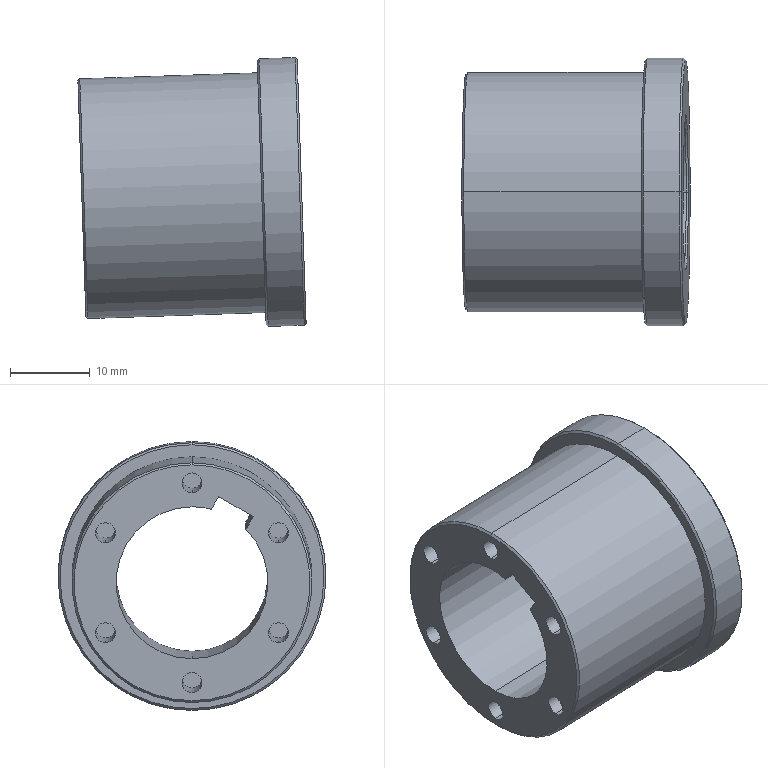Part | STEP file | 2026.6.15-Main Assembly图.sldasm-Part-99 | 1 solid | 40 faces | box 28.541 x 33.5 x 33.633 mm | volume 11781 mm3 | cylinder 19 | plane 12 | cone 9 | commonest cylinder face diameters 2.5 x12 19 x3 30 x2 33.5 x2
STEP:
#1=CARTESIAN_POINT('',(-1536.134,735.086,4103.375));
#2=VERTEX_POINT('',#1);
#3=CARTESIAN_POINT('',(-1537.25,735.086,4136.356));
#4=VERTEX_POINT('',#3);
#5=CARTESIAN_POINT('',(-1536.692,735.086,4119.866));
#6=DIRECTION('',(0.9994,0.,0.03381));
#7=DIRECTION('',(0.03381,0.,-0.9994));
#8=AXIS2_PLACEMENT_3D('',#5,#6,#7);
#9=CIRCLE('',#8,16.5);
#10=EDGE_CURVE('',#2,#4,#9,.T.);
#11=ORIENTED_EDGE('',*,*,#10,.F.);
#12=CARTESIAN_POINT('',(-1536.375,735.086,4103.117));
#13=VERTEX_POINT('',#12);
#14=CARTESIAN_POINT('',(-1536.134,735.086,4103.375));
#15=DIRECTION('',(-0.6828,0.,-0.7306));
#16=VECTOR('',#15,1000.);
#17=LINE('',#14,#16);
#18=EDGE_CURVE('',#2,#13,#17,.T.);
#19=ORIENTED_EDGE('',*,*,#18,.T.);
#20=CARTESIAN_POINT('',(-1537.508,735.086,4136.598));
#21=VERTEX_POINT('',#20);
#22=CARTESIAN_POINT('',(-1536.941,735.086,4119.857));
#23=DIRECTION('',(-0.9994,0.,-0.03381));
#24=DIRECTION('',(0.03381,0.,-0.9994));
#25=AXIS2_PLACEMENT_3D('',#22,#23,#24);
#26=CIRCLE('',#25,16.75);
#27=EDGE_CURVE('',#21,#13,#26,.T.);
#28=ORIENTED_EDGE('',*,*,#27,.F.);
#29=CARTESIAN_POINT('',(-1537.25,735.086,4136.356));
#30=DIRECTION('',(-0.7306,0.,0.6828));
#31=VECTOR('',#30,1000.);
#32=LINE('',#29,#31);
#33=EDGE_CURVE('',#4,#21,#32,.T.);
#34=ORIENTED_EDGE('',*,*,#33,.F.);
#35=EDGE_LOOP('',(#11,#19,#28,#34));
#36=FACE_OUTER_BOUND('',#35,.T.);
#37=CARTESIAN_POINT('',(-1536.692,735.086,4119.866));
#38=DIRECTION('',(-0.9994,0.,-0.03381));
#39=DIRECTION('',(-0.03381,0.,0.9994));
#40=AXIS2_PLACEMENT_3D('',#37,#38,#39);
#41=CONICAL_SURFACE('',#40,16.5,0.7854);
#42=ADVANCED_FACE('',(#36),#41,.T.);
#43=CARTESIAN_POINT('',(-1542.247,735.086,4136.187));
#44=VERTEX_POINT('',#43);
#45=CARTESIAN_POINT('',(-1541.131,735.086,4103.206));
#46=VERTEX_POINT('',#45);
#47=CARTESIAN_POINT('',(-1541.689,735.086,4119.697));
#48=DIRECTION('',(-0.9994,0.,-0.03381));
#49=DIRECTION('',(0.03381,0.,-0.9994));
#50=AXIS2_PLACEMENT_3D('',#47,#48,#49);
#51=CIRCLE('',#50,16.5);
#52=EDGE_CURVE('',#44,#46,#51,.T.);
#53=ORIENTED_EDGE('',*,*,#52,.F.);
#54=CARTESIAN_POINT('',(-1542.005,735.086,4136.445));
#55=VERTEX_POINT('',#54);
#56=CARTESIAN_POINT('',(-1542.005,735.086,4136.445));
#57=DIRECTION('',(0.6828,0.,0.7306));
#58=VECTOR('',#57,1000.);
#59=LINE('',#56,#58);
#60=EDGE_CURVE('',#44,#55,#59,.T.);
#61=ORIENTED_EDGE('',*,*,#60,.T.);
#62=CARTESIAN_POINT('',(-1540.873,735.086,4102.965));
#63=VERTEX_POINT('',#62);
#64=CARTESIAN_POINT('',(-1541.439,735.086,4119.705));
#65=DIRECTION('',(0.9994,0.,0.03381));
#66=DIRECTION('',(0.03381,0.,-0.9994));
#67=AXIS2_PLACEMENT_3D('',#64,#65,#66);
#68=CIRCLE('',#67,16.75);
#69=EDGE_CURVE('',#63,#55,#68,.T.);
#70=ORIENTED_EDGE('',*,*,#69,.F.);
#71=CARTESIAN_POINT('',(-1540.873,735.086,4102.965));
#72=DIRECTION('',(0.7306,0.,-0.6828));
#73=VECTOR('',#72,1000.);
#74=LINE('',#71,#73);
#75=EDGE_CURVE('',#46,#63,#74,.T.);
#76=ORIENTED_EDGE('',*,*,#75,.F.);
#77=EDGE_LOOP('',(#53,#61,#70,#76));
#78=FACE_OUTER_BOUND('',#77,.T.);
#79=CARTESIAN_POINT('',(-1541.439,735.086,4119.705));
#80=DIRECTION('',(0.9994,0.,0.03381));
#81=DIRECTION('',(0.03381,0.,-0.9994));
#82=AXIS2_PLACEMENT_3D('',#79,#80,#81);
#83=CONICAL_SURFACE('',#82,16.75,0.7854);
#84=ADVANCED_FACE('',(#78),#83,.T.);
#85=CARTESIAN_POINT('',(-1537.263,735.086,4129.352));
#86=VERTEX_POINT('',#85);
#87=CARTESIAN_POINT('',(-1537.252,732.668,4129.039));
#88=VERTEX_POINT('',#87);
#89=CARTESIAN_POINT('',(-1536.941,735.086,4119.857));
#90=DIRECTION('',(0.9994,0.,0.03381));
#91=DIRECTION('',(0.03381,0.,-0.9994));
#92=AXIS2_PLACEMENT_3D('',#89,#90,#91);
#93=CIRCLE('',#92,9.5);
#94=EDGE_CURVE('',#86,#88,#93,.T.);
#95=ORIENTED_EDGE('',*,*,#94,.F.);
#96=CARTESIAN_POINT('',(-1537.021,735.086,4129.61));
#97=VERTEX_POINT('',#96);
#98=CARTESIAN_POINT('',(-1537.263,735.086,4129.352));
#99=DIRECTION('',(0.6828,0.,0.7306));
#100=VECTOR('',#99,1000.);
#101=LINE('',#98,#100);
#102=EDGE_CURVE('',#86,#97,#101,.T.);
#103=ORIENTED_EDGE('',*,*,#102,.T.);
#104=CARTESIAN_POINT('',(-1537.01,732.539,4129.272));
#105=VERTEX_POINT('',#104);
#106=CARTESIAN_POINT('',(-1536.692,735.086,4119.866));
#107=DIRECTION('',(-0.9994,0.,-0.03381));
#108=DIRECTION('',(0.03381,0.,-0.9994));
#109=AXIS2_PLACEMENT_3D('',#106,#107,#108);
#110=CIRCLE('',#109,9.75);
#111=EDGE_CURVE('',#105,#97,#110,.T.);
#112=ORIENTED_EDGE('',*,*,#111,.F.);
#113=CARTESIAN_POINT('',(-1537.252,732.668,4129.039));
#114=CARTESIAN_POINT('',(-1537.171,732.625,4129.117));
#115=CARTESIAN_POINT('',(-1537.091,732.582,4129.194));
#116=CARTESIAN_POINT('',(-1537.01,732.539,4129.272));
#117=B_SPLINE_CURVE_WITH_KNOTS('',3,(#113,#114,#115,#116),.UNSPECIFIED.,.F.,.F.,(4,4),(0.,0.0003599),.UNSPECIFIED.);
#118=EDGE_CURVE('',#88,#105,#117,.T.);
#119=ORIENTED_EDGE('',*,*,#118,.F.);
#120=EDGE_LOOP('',(#95,#103,#112,#119));
#121=FACE_OUTER_BOUND('',#120,.T.);
#122=CARTESIAN_POINT('',(-1536.941,735.086,4119.857));
#123=DIRECTION('',(0.9994,0.,0.03381));
#124=DIRECTION('',(0.03381,0.,-0.9994));
#125=AXIS2_PLACEMENT_3D('',#122,#123,#124);
#126=CONICAL_SURFACE('',#125,9.5,0.7854);
#127=ADVANCED_FACE('',(#121),#126,.F.);
#128=ORIENTED_EDGE('',*,*,#102,.F.);
#129=CARTESIAN_POINT('',(-1536.62,735.086,4110.363));
#130=VERTEX_POINT('',#129);
#131=CARTESIAN_POINT('',(-1536.941,735.086,4119.857));
#132=DIRECTION('',(0.9994,0.,0.03381));
#133=DIRECTION('',(0.03381,0.,-0.9994));
#134=AXIS2_PLACEMENT_3D('',#131,#132,#133);
#135=CIRCLE('',#134,9.5);
#136=EDGE_CURVE('',#130,#86,#135,.T.);
#137=ORIENTED_EDGE('',*,*,#136,.F.);
#138=CARTESIAN_POINT('',(-1536.362,735.086,4110.121));
#139=VERTEX_POINT('',#138);
#140=CARTESIAN_POINT('',(-1536.62,735.086,4110.363));
#141=DIRECTION('',(0.7306,0.,-0.6828));
#142=VECTOR('',#141,1000.);
#143=LINE('',#140,#142);
#144=EDGE_CURVE('',#130,#139,#143,.T.);
#145=ORIENTED_EDGE('',*,*,#144,.T.);
#146=CARTESIAN_POINT('',(-1536.692,735.086,4119.866));
#147=DIRECTION('',(-0.9994,0.,-0.03381));
#148=DIRECTION('',(0.03381,0.,-0.9994));
#149=AXIS2_PLACEMENT_3D('',#146,#147,#148);
#150=CIRCLE('',#149,9.75);
#151=EDGE_CURVE('',#97,#139,#150,.T.);
#152=ORIENTED_EDGE('',*,*,#151,.F.);
#153=EDGE_LOOP('',(#128,#137,#145,#152));
#154=FACE_OUTER_BOUND('',#153,.T.);
#155=CARTESIAN_POINT('',(-1536.941,735.086,4119.857));
#156=DIRECTION('',(0.9994,0.,0.03381));
#157=DIRECTION('',(0.03381,0.,-0.9994));
#158=AXIS2_PLACEMENT_3D('',#155,#156,#157);
#159=CONICAL_SURFACE('',#158,9.5,0.7854);
#160=ADVANCED_FACE('',(#154),#159,.F.);
#161=CARTESIAN_POINT('',(-1564.675,735.086,4133.677));
#162=VERTEX_POINT('',#161);
#163=CARTESIAN_POINT('',(-1563.677,735.086,4104.194));
#164=VERTEX_POINT('',#163);
#165=CARTESIAN_POINT('',(-1564.176,735.086,4118.936));
#166=DIRECTION('',(-0.9994,0.,-0.03381));
#167=DIRECTION('',(0.03381,0.,-0.9994));
#168=AXIS2_PLACEMENT_3D('',#165,#166,#167);
#169=CIRCLE('',#168,14.75);
#170=EDGE_CURVE('',#162,#164,#169,.T.);
#171=ORIENTED_EDGE('',*,*,#170,.F.);
#172=CARTESIAN_POINT('',(-1564.433,735.086,4133.936));
#173=VERTEX_POINT('',#172);
#174=CARTESIAN_POINT('',(-1564.433,735.086,4133.936));
#175=DIRECTION('',(0.6828,0.,0.7306));
#176=VECTOR('',#175,1000.);
#177=LINE('',#174,#176);
#178=EDGE_CURVE('',#162,#173,#177,.T.);
#179=ORIENTED_EDGE('',*,*,#178,.T.);
#180=CARTESIAN_POINT('',(-1563.419,735.086,4103.953));
#181=VERTEX_POINT('',#180);
#182=CARTESIAN_POINT('',(-1563.926,735.086,4118.944));
#183=DIRECTION('',(0.9994,0.,0.03381));
#184=DIRECTION('',(0.03381,0.,-0.9994));
#185=AXIS2_PLACEMENT_3D('',#182,#183,#184);
#186=CIRCLE('',#185,15.);
#187=EDGE_CURVE('',#181,#173,#186,.T.);
#188=ORIENTED_EDGE('',*,*,#187,.F.);
#189=CARTESIAN_POINT('',(-1563.419,735.086,4103.953));
#190=DIRECTION('',(0.7306,0.,-0.6828));
#191=VECTOR('',#190,1000.);
#192=LINE('',#189,#191);
#193=EDGE_CURVE('',#164,#181,#192,.T.);
#194=ORIENTED_EDGE('',*,*,#193,.F.);
#195=EDGE_LOOP('',(#171,#179,#188,#194));
#196=FACE_OUTER_BOUND('',#195,.T.);
#197=CARTESIAN_POINT('',(-1563.926,735.086,4118.944));
#198=DIRECTION('',(0.9994,0.,0.03381));
#199=DIRECTION('',(0.03381,0.,-0.9994));
#200=AXIS2_PLACEMENT_3D('',#197,#198,#199);
#201=CONICAL_SURFACE('',#200,15.,0.7854);
#202=ADVANCED_FACE('',(#196),#201,.T.);
#203=CARTESIAN_POINT('',(-1564.556,735.086,4130.179));
#204=VERTEX_POINT('',#203);
#205=CARTESIAN_POINT('',(-1564.641,735.086,4132.678));
#206=VERTEX_POINT('',#205);
#207=CARTESIAN_POINT('',(-1564.599,735.086,4131.429));
#208=DIRECTION('',(-0.9994,0.,-0.03381));
#209=DIRECTION('',(-0.02928,-0.5,0.8655));
#210=AXIS2_PLACEMENT_3D('',#207,#208,#209);
#211=CIRCLE('',#210,1.25);
#212=EDGE_CURVE('',#204,#206,#211,.T.);
#213=ORIENTED_EDGE('',*,*,#212,.T.);
#214=CARTESIAN_POINT('',(-1547.651,735.086,4133.253));
#215=VERTEX_POINT('',#214);
#216=CARTESIAN_POINT('',(-1564.641,735.086,4132.678));
#217=DIRECTION('',(0.9994,0.,0.03381));
#218=VECTOR('',#217,1000.);
#219=LINE('',#216,#218);
#220=EDGE_CURVE('',#206,#215,#219,.T.);
#221=ORIENTED_EDGE('',*,*,#220,.T.);
#222=CARTESIAN_POINT('',(-1547.566,735.086,4130.754));
#223=VERTEX_POINT('',#222);
#224=CARTESIAN_POINT('',(-1547.608,735.086,4132.003));
#225=DIRECTION('',(0.9994,0.,0.03381));
#226=DIRECTION('',(-0.02928,-0.5,0.8655));
#227=AXIS2_PLACEMENT_3D('',#224,#225,#226);
#228=CIRCLE('',#227,1.25);
#229=EDGE_CURVE('',#215,#223,#228,.T.);
#230=ORIENTED_EDGE('',*,*,#229,.T.);
#231=CARTESIAN_POINT('',(-1564.556,735.086,4130.179));
#232=DIRECTION('',(0.9994,0.,0.03381));
#233=VECTOR('',#232,1000.);
#234=LINE('',#231,#233);
#235=EDGE_CURVE('',#204,#223,#234,.T.);
#236=ORIENTED_EDGE('',*,*,#235,.F.);
#237=EDGE_LOOP('',(#213,#221,#230,#236));
#238=FACE_OUTER_BOUND('',#237,.T.);
#239=CARTESIAN_POINT('',(-1564.599,735.086,4131.429));
#240=DIRECTION('',(0.9994,0.,0.03381));
#241=DIRECTION('',(0.03381,0.,-0.9994));
#242=AXIS2_PLACEMENT_3D('',#239,#240,#241);
#243=CYLINDRICAL_SURFACE('',#242,1.25);
#244=ADVANCED_FACE('',(#238),#243,.F.);
#245=CARTESIAN_POINT('',(-1564.345,724.26,4123.933));
#246=VERTEX_POINT('',#245);
#247=CARTESIAN_POINT('',(-1564.429,724.26,4126.431));
#248=VERTEX_POINT('',#247);
#249=CARTESIAN_POINT('',(-1564.387,724.26,4125.182));
#250=DIRECTION('',(-0.9994,0.,-0.03381));
#251=DIRECTION('',(-0.02928,-0.5,0.8655));
#252=AXIS2_PLACEMENT_3D('',#249,#250,#251);
#253=CIRCLE('',#252,1.25);
#254=EDGE_CURVE('',#246,#248,#253,.T.);
#255=ORIENTED_EDGE('',*,*,#254,.T.);
#256=CARTESIAN_POINT('',(-1547.439,724.26,4127.006));
#257=VERTEX_POINT('',#256);
#258=CARTESIAN_POINT('',(-1564.429,724.26,4126.431));
#259=DIRECTION('',(0.9994,0.,0.03381));
#260=VECTOR('',#259,1000.);
#261=LINE('',#258,#260);
#262=EDGE_CURVE('',#248,#257,#261,.T.);
#263=ORIENTED_EDGE('',*,*,#262,.T.);
#264=CARTESIAN_POINT('',(-1547.355,724.26,4124.508));
#265=VERTEX_POINT('',#264);
#266=CARTESIAN_POINT('',(-1547.397,724.26,4125.757));
#267=DIRECTION('',(0.9994,0.,0.03381));
#268=DIRECTION('',(-0.02928,-0.5,0.8655));
#269=AXIS2_PLACEMENT_3D('',#266,#267,#268);
#270=CIRCLE('',#269,1.25);
#271=EDGE_CURVE('',#257,#265,#270,.T.);
#272=ORIENTED_EDGE('',*,*,#271,.T.);
#273=CARTESIAN_POINT('',(-1564.345,724.26,4123.933));
#274=DIRECTION('',(0.9994,0.,0.03381));
#275=VECTOR('',#274,1000.);
#276=LINE('',#273,#275);
#277=EDGE_CURVE('',#246,#265,#276,.T.);
#278=ORIENTED_EDGE('',*,*,#277,.F.);
#279=EDGE_LOOP('',(#255,#263,#272,#278));
#280=FACE_OUTER_BOUND('',#279,.T.);
#281=CARTESIAN_POINT('',(-1564.387,724.26,4125.182));
#282=DIRECTION('',(0.9994,0.,0.03381));
#283=DIRECTION('',(0.03381,0.,-0.9994));
#284=AXIS2_PLACEMENT_3D('',#281,#282,#283);
#285=CYLINDRICAL_SURFACE('',#284,1.25);
#286=ADVANCED_FACE('',(#280),#285,.F.);
#287=CARTESIAN_POINT('',(-1563.922,724.26,4111.44));
#288=VERTEX_POINT('',#287);
#289=CARTESIAN_POINT('',(-1564.007,724.26,4113.939));
#290=VERTEX_POINT('',#289);
#291=CARTESIAN_POINT('',(-1563.965,724.26,4112.689));
#292=DIRECTION('',(-0.9994,0.,-0.03381));
#293=DIRECTION('',(-0.02928,-0.5,0.8655));
#294=AXIS2_PLACEMENT_3D('',#291,#292,#293);
#295=CIRCLE('',#294,1.25);
#296=EDGE_CURVE('',#288,#290,#295,.T.);
#297=ORIENTED_EDGE('',*,*,#296,.T.);
#298=CARTESIAN_POINT('',(-1547.017,724.26,4114.513));
#299=VERTEX_POINT('',#298);
#300=CARTESIAN_POINT('',(-1564.007,724.26,4113.939));
#301=DIRECTION('',(0.9994,0.,0.03381));
#302=VECTOR('',#301,1000.);
#303=LINE('',#300,#302);
#304=EDGE_CURVE('',#290,#299,#303,.T.);
#305=ORIENTED_EDGE('',*,*,#304,.T.);
#306=CARTESIAN_POINT('',(-1546.932,724.26,4112.015));
#307=VERTEX_POINT('',#306);
#308=CARTESIAN_POINT('',(-1546.974,724.26,4113.264));
#309=DIRECTION('',(0.9994,0.,0.03381));
#310=DIRECTION('',(-0.02928,-0.5,0.8655));
#311=AXIS2_PLACEMENT_3D('',#308,#309,#310);
#312=CIRCLE('',#311,1.25);
#313=EDGE_CURVE('',#299,#307,#312,.T.);
#314=ORIENTED_EDGE('',*,*,#313,.T.);
#315=CARTESIAN_POINT('',(-1563.922,724.26,4111.44));
#316=DIRECTION('',(0.9994,0.,0.03381));
#317=VECTOR('',#316,1000.);
#318=LINE('',#315,#317);
#319=EDGE_CURVE('',#288,#307,#318,.T.);
#320=ORIENTED_EDGE('',*,*,#319,.F.);
#321=EDGE_LOOP('',(#297,#305,#314,#320));
#322=FACE_OUTER_BOUND('',#321,.T.);
#323=CARTESIAN_POINT('',(-1563.965,724.26,4112.689));
#324=DIRECTION('',(0.9994,0.,0.03381));
#325=DIRECTION('',(0.03381,0.,-0.9994));
#326=AXIS2_PLACEMENT_3D('',#323,#324,#325);
#327=CYLINDRICAL_SURFACE('',#326,1.25);
#328=ADVANCED_FACE('',(#322),#327,.F.);
#329=CARTESIAN_POINT('',(-1563.711,735.086,4105.194));
#330=VERTEX_POINT('',#329);
#331=CARTESIAN_POINT('',(-1563.795,735.086,4107.692));
#332=VERTEX_POINT('',#331);
#333=CARTESIAN_POINT('',(-1563.753,735.086,4106.443));
#334=DIRECTION('',(-0.9994,0.,-0.03381));
#335=DIRECTION('',(-0.02928,-0.5,0.8655));
#336=AXIS2_PLACEMENT_3D('',#333,#334,#335);
#337=CIRCLE('',#336,1.25);
#338=EDGE_CURVE('',#330,#332,#337,.T.);
#339=ORIENTED_EDGE('',*,*,#338,.T.);
#340=CARTESIAN_POINT('',(-1546.805,735.086,4108.267));
#341=VERTEX_POINT('',#340);
#342=CARTESIAN_POINT('',(-1563.795,735.086,4107.692));
#343=DIRECTION('',(0.9994,0.,0.03381));
#344=VECTOR('',#343,1000.);
#345=LINE('',#342,#344);
#346=EDGE_CURVE('',#332,#341,#345,.T.);
#347=ORIENTED_EDGE('',*,*,#346,.T.);
#348=CARTESIAN_POINT('',(-1546.721,735.086,4105.768));
#349=VERTEX_POINT('',#348);
#350=CARTESIAN_POINT('',(-1546.763,735.086,4107.018));
#351=DIRECTION('',(0.9994,0.,0.03381));
#352=DIRECTION('',(-0.02928,-0.5,0.8655));
#353=AXIS2_PLACEMENT_3D('',#350,#351,#352);
#354=CIRCLE('',#353,1.25);
#355=EDGE_CURVE('',#341,#349,#354,.T.);
#356=ORIENTED_EDGE('',*,*,#355,.T.);
#357=CARTESIAN_POINT('',(-1563.711,735.086,4105.194));
#358=DIRECTION('',(0.9994,0.,0.03381));
#359=VECTOR('',#358,1000.);
#360=LINE('',#357,#359);
#361=EDGE_CURVE('',#330,#349,#360,.T.);
#362=ORIENTED_EDGE('',*,*,#361,.F.);
#363=EDGE_LOOP('',(#339,#347,#356,#362));
#364=FACE_OUTER_BOUND('',#363,.T.);
#365=CARTESIAN_POINT('',(-1563.753,735.086,4106.443));
#366=DIRECTION('',(0.9994,0.,0.03381));
#367=DIRECTION('',(0.03381,0.,-0.9994));
#368=AXIS2_PLACEMENT_3D('',#365,#366,#367);
#369=CYLINDRICAL_SURFACE('',#368,1.25);
#370=ADVANCED_FACE('',(#364),#369,.F.);
#371=CARTESIAN_POINT('',(-1563.922,745.911,4111.44));
#372=VERTEX_POINT('',#371);
#373=CARTESIAN_POINT('',(-1564.007,745.911,4113.939));
#374=VERTEX_POINT('',#373);
#375=CARTESIAN_POINT('',(-1563.965,745.911,4112.689));
#376=DIRECTION('',(-0.9994,0.,-0.03381));
#377=DIRECTION('',(-0.02928,-0.5,0.8655));
#378=AXIS2_PLACEMENT_3D('',#375,#376,#377);
#379=CIRCLE('',#378,1.25);
#380=EDGE_CURVE('',#372,#374,#379,.T.);
#381=ORIENTED_EDGE('',*,*,#380,.T.);
#382=CARTESIAN_POINT('',(-1547.017,745.911,4114.513));
#383=VERTEX_POINT('',#382);
#384=CARTESIAN_POINT('',(-1564.007,745.911,4113.939));
#385=DIRECTION('',(0.9994,0.,0.03381));
#386=VECTOR('',#385,1000.);
#387=LINE('',#384,#386);
#388=EDGE_CURVE('',#374,#383,#387,.T.);
#389=ORIENTED_EDGE('',*,*,#388,.T.);
#390=CARTESIAN_POINT('',(-1546.932,745.911,4112.015));
#391=VERTEX_POINT('',#390);
#392=CARTESIAN_POINT('',(-1546.974,745.911,4113.264));
#393=DIRECTION('',(0.9994,0.,0.03381));
#394=DIRECTION('',(-0.02928,-0.5,0.8655));
#395=AXIS2_PLACEMENT_3D('',#392,#393,#394);
#396=CIRCLE('',#395,1.25);
#397=EDGE_CURVE('',#383,#391,#396,.T.);
#398=ORIENTED_EDGE('',*,*,#397,.T.);
#399=CARTESIAN_POINT('',(-1563.922,745.911,4111.44));
#400=DIRECTION('',(0.9994,0.,0.03381));
#401=VECTOR('',#400,1000.);
#402=LINE('',#399,#401);
#403=EDGE_CURVE('',#372,#391,#402,.T.);
#404=ORIENTED_EDGE('',*,*,#403,.F.);
#405=EDGE_LOOP('',(#381,#389,#398,#404));
#406=FACE_OUTER_BOUND('',#405,.T.);
#407=CARTESIAN_POINT('',(-1563.965,745.911,4112.689));
#408=DIRECTION('',(0.9994,0.,0.03381));
#409=DIRECTION('',(0.03381,0.,-0.9994));
#410=AXIS2_PLACEMENT_3D('',#407,#408,#409);
#411=CYLINDRICAL_SURFACE('',#410,1.25);
#412=ADVANCED_FACE('',(#406),#411,.F.);
#413=CARTESIAN_POINT('',(-1564.345,745.911,4123.933));
#414=VERTEX_POINT('',#413);
#415=CARTESIAN_POINT('',(-1564.429,745.911,4126.431));
#416=VERTEX_POINT('',#415);
#417=CARTESIAN_POINT('',(-1564.387,745.911,4125.182));
#418=DIRECTION('',(-0.9994,0.,-0.03381));
#419=DIRECTION('',(-0.02928,-0.5,0.8655));
#420=AXIS2_PLACEMENT_3D('',#417,#418,#419);
#421=CIRCLE('',#420,1.25);
#422=EDGE_CURVE('',#414,#416,#421,.T.);
#423=ORIENTED_EDGE('',*,*,#422,.T.);
#424=CARTESIAN_POINT('',(-1547.439,745.911,4127.006));
#425=VERTEX_POINT('',#424);
#426=CARTESIAN_POINT('',(-1564.429,745.911,4126.431));
#427=DIRECTION('',(0.9994,0.,0.03381));
#428=VECTOR('',#427,1000.);
#429=LINE('',#426,#428);
#430=EDGE_CURVE('',#416,#425,#429,.T.);
#431=ORIENTED_EDGE('',*,*,#430,.T.);
#432=CARTESIAN_POINT('',(-1547.355,745.911,4124.508));
#433=VERTEX_POINT('',#432);
#434=CARTESIAN_POINT('',(-1547.397,745.911,4125.757));
#435=DIRECTION('',(0.9994,0.,0.03381));
#436=DIRECTION('',(-0.02928,-0.5,0.8655));
#437=AXIS2_PLACEMENT_3D('',#434,#435,#436);
#438=CIRCLE('',#437,1.25);
#439=EDGE_CURVE('',#425,#433,#438,.T.);
#440=ORIENTED_EDGE('',*,*,#439,.T.);
#441=CARTESIAN_POINT('',(-1564.345,745.911,4123.933));
#442=DIRECTION('',(0.9994,0.,0.03381));
#443=VECTOR('',#442,1000.);
#444=LINE('',#441,#443);
#445=EDGE_CURVE('',#414,#433,#444,.T.);
#446=ORIENTED_EDGE('',*,*,#445,.F.);
#447=EDGE_LOOP('',(#423,#431,#440,#446));
#448=FACE_OUTER_BOUND('',#447,.T.);
#449=CARTESIAN_POINT('',(-1564.387,745.911,4125.182));
#450=DIRECTION('',(0.9994,0.,0.03381));
#451=DIRECTION('',(0.03381,0.,-0.9994));
#452=AXIS2_PLACEMENT_3D('',#449,#450,#451);
#453=CYLINDRICAL_SURFACE('',#452,1.25);
#454=ADVANCED_FACE('',(#448),#453,.F.);
#455=CARTESIAN_POINT('',(-1564.497,735.086,4128.43));
#456=VERTEX_POINT('',#455);
#457=CARTESIAN_POINT('',(-1564.487,732.668,4128.118));
#458=VERTEX_POINT('',#457);
#459=CARTESIAN_POINT('',(-1564.176,735.086,4118.936));
#460=DIRECTION('',(0.9994,0.,0.03381));
#461=DIRECTION('',(-0.01691,0.866,0.4997));
#462=AXIS2_PLACEMENT_3D('',#459,#460,#461);
#463=CIRCLE('',#462,9.5);
#464=EDGE_CURVE('',#456,#458,#463,.T.);
#465=ORIENTED_EDGE('',*,*,#464,.F.);
#466=CARTESIAN_POINT('',(-1564.497,735.086,4128.43));
#467=DIRECTION('',(0.9994,0.,0.03381));
#468=VECTOR('',#467,1000.);
#469=LINE('',#466,#468);
#470=EDGE_CURVE('',#456,#86,#469,.T.);
#471=ORIENTED_EDGE('',*,*,#470,.T.);
#472=ORIENTED_EDGE('',*,*,#94,.T.);
#473=CARTESIAN_POINT('',(-1564.487,732.668,4128.118));
#474=DIRECTION('',(-0.9994,0.,-0.03381));
#475=VECTOR('',#474,1000.);
#476=LINE('',#473,#475);
#477=EDGE_CURVE('',#88,#458,#476,.T.);
#478=ORIENTED_EDGE('',*,*,#477,.T.);
#479=EDGE_LOOP('',(#465,#471,#472,#478));
#480=FACE_OUTER_BOUND('',#479,.T.);
#481=CARTESIAN_POINT('',(-1564.176,735.086,4118.936));
#482=DIRECTION('',(0.9994,0.,0.03381));
#483=DIRECTION('',(0.03381,0.,-0.9994));
#484=AXIS2_PLACEMENT_3D('',#481,#482,#483);
#485=CYLINDRICAL_SURFACE('',#484,9.5);
#486=ADVANCED_FACE('',(#480),#485,.F.);
#487=ORIENTED_EDGE('',*,*,#470,.F.);
#488=CARTESIAN_POINT('',(-1563.855,735.086,4109.441));
#489=VERTEX_POINT('',#488);
#490=CARTESIAN_POINT('',(-1564.176,735.086,4118.936));
#491=DIRECTION('',(0.9994,0.,0.03381));
#492=DIRECTION('',(-0.01691,0.866,0.4997));
#493=AXIS2_PLACEMENT_3D('',#490,#491,#492);
#494=CIRCLE('',#493,9.5);
#495=EDGE_CURVE('',#489,#456,#494,.T.);
#496=ORIENTED_EDGE('',*,*,#495,.F.);
#497=CARTESIAN_POINT('',(-1563.855,735.086,4109.441));
#498=DIRECTION('',(0.9994,0.,0.03381));
#499=VECTOR('',#498,1000.);
#500=LINE('',#497,#499);
#501=EDGE_CURVE('',#489,#130,#500,.T.);
#502=ORIENTED_EDGE('',*,*,#501,.T.);
#503=ORIENTED_EDGE('',*,*,#136,.T.);
#504=EDGE_LOOP('',(#487,#496,#502,#503));
#505=FACE_OUTER_BOUND('',#504,.T.);
#506=CARTESIAN_POINT('',(-1564.176,735.086,4118.936));
#507=DIRECTION('',(0.9994,0.,0.03381));
#508=DIRECTION('',(0.03381,0.,-0.9994));
#509=AXIS2_PLACEMENT_3D('',#506,#507,#508);
#510=CYLINDRICAL_SURFACE('',#509,9.5);
#511=ADVANCED_FACE('',(#505),#510,.F.);
#512=ORIENTED_EDGE('',*,*,#187,.T.);
#513=CARTESIAN_POINT('',(-1542.196,735.086,4134.688));
#514=VERTEX_POINT('',#513);
#515=CARTESIAN_POINT('',(-1564.683,735.086,4133.927));
#516=DIRECTION('',(0.9994,0.,0.03381));
#517=VECTOR('',#516,1000.);
#518=LINE('',#515,#517);
#519=EDGE_CURVE('',#173,#514,#518,.T.);
#520=ORIENTED_EDGE('',*,*,#519,.T.);
#521=CARTESIAN_POINT('',(-1541.182,735.086,4104.705));
#522=VERTEX_POINT('',#521);
#523=CARTESIAN_POINT('',(-1541.689,735.086,4119.697));
#524=DIRECTION('',(0.9994,0.,0.03381));
#525=DIRECTION('',(0.03381,0.,-0.9994));
#526=AXIS2_PLACEMENT_3D('',#523,#524,#525);
#527=CIRCLE('',#526,15.);
#528=EDGE_CURVE('',#522,#514,#527,.T.);
#529=ORIENTED_EDGE('',*,*,#528,.F.);
#530=CARTESIAN_POINT('',(-1563.669,735.086,4103.944));
#531=DIRECTION('',(0.9994,0.,0.03381));
#532=VECTOR('',#531,1000.);
#533=LINE('',#530,#532);
#534=EDGE_CURVE('',#181,#522,#533,.T.);
#535=ORIENTED_EDGE('',*,*,#534,.F.);
#536=EDGE_LOOP('',(#512,#520,#529,#535));
#537=FACE_OUTER_BOUND('',#536,.T.);
#538=CARTESIAN_POINT('',(-1564.176,735.086,4118.936));
#539=DIRECTION('',(0.9994,0.,0.03381));
#540=DIRECTION('',(0.03381,0.,-0.9994));
#541=AXIS2_PLACEMENT_3D('',#538,#539,#540);
#542=CYLINDRICAL_SURFACE('',#541,15.);
#543=ADVANCED_FACE('',(#537),#542,.T.);
#544=ORIENTED_EDGE('',*,*,#69,.T.);
#545=CARTESIAN_POINT('',(-1542.255,735.086,4136.437));
#546=DIRECTION('',(0.9994,0.,0.03381));
#547=VECTOR('',#546,1000.);
#548=LINE('',#545,#547);
#549=EDGE_CURVE('',#55,#21,#548,.T.);
#550=ORIENTED_EDGE('',*,*,#549,.T.);
#551=ORIENTED_EDGE('',*,*,#27,.T.);
#552=CARTESIAN_POINT('',(-1541.122,735.086,4102.956));
#553=DIRECTION('',(0.9994,0.,0.03381));
#554=VECTOR('',#553,1000.);
#555=LINE('',#552,#554);
#556=EDGE_CURVE('',#63,#13,#555,.T.);
#557=ORIENTED_EDGE('',*,*,#556,.F.);
#558=EDGE_LOOP('',(#544,#550,#551,#557));
#559=FACE_OUTER_BOUND('',#558,.T.);
#560=CARTESIAN_POINT('',(-1541.689,735.086,4119.697));
#561=DIRECTION('',(0.9994,0.,0.03381));
#562=DIRECTION('',(0.03381,0.,-0.9994));
#563=AXIS2_PLACEMENT_3D('',#560,#561,#562);
#564=CYLINDRICAL_SURFACE('',#563,16.75);
#565=ADVANCED_FACE('',(#559),#564,.T.);
#566=ORIENTED_EDGE('',*,*,#549,.F.);
#567=CARTESIAN_POINT('',(-1541.439,735.086,4119.705));
#568=DIRECTION('',(0.9994,0.,0.03381));
#569=DIRECTION('',(0.03381,0.,-0.9994));
#570=AXIS2_PLACEMENT_3D('',#567,#568,#569);
#571=CIRCLE('',#570,16.75);
#572=EDGE_CURVE('',#55,#63,#571,.T.);
#573=ORIENTED_EDGE('',*,*,#572,.T.);
#574=ORIENTED_EDGE('',*,*,#556,.T.);
#575=CARTESIAN_POINT('',(-1536.941,735.086,4119.857));
#576=DIRECTION('',(-0.9994,0.,-0.03381));
#577=DIRECTION('',(0.03381,0.,-0.9994));
#578=AXIS2_PLACEMENT_3D('',#575,#576,#577);
#579=CIRCLE('',#578,16.75);
#580=EDGE_CURVE('',#13,#21,#579,.T.);
#581=ORIENTED_EDGE('',*,*,#580,.T.);
#582=EDGE_LOOP('',(#566,#573,#574,#581));
#583=FACE_OUTER_BOUND('',#582,.T.);
#584=CARTESIAN_POINT('',(-1541.689,735.086,4119.697));
#585=DIRECTION('',(0.9994,0.,0.03381));
#586=DIRECTION('',(0.03381,0.,-0.9994));
#587=AXIS2_PLACEMENT_3D('',#584,#585,#586);
#588=CYLINDRICAL_SURFACE('',#587,16.75);
#589=ADVANCED_FACE('',(#583),#588,.T.);
#590=CARTESIAN_POINT('',(-1541.689,735.086,4119.697));
#591=DIRECTION('',(-0.9994,0.,-0.03381));
#592=DIRECTION('',(0.03381,0.,-0.9994));
#593=AXIS2_PLACEMENT_3D('',#590,#591,#592);
#594=CIRCLE('',#593,16.5);
#595=EDGE_CURVE('',#46,#44,#594,.T.);
#596=ORIENTED_EDGE('',*,*,#595,.T.);
#597=ORIENTED_EDGE('',*,*,#52,.T.);
#598=EDGE_LOOP('',(#596,#597));
#599=FACE_OUTER_BOUND('',#598,.T.);
#600=ORIENTED_EDGE('',*,*,#528,.T.);
#601=CARTESIAN_POINT('',(-1541.689,735.086,4119.697));
#602=DIRECTION('',(0.9994,0.,0.03381));
#603=DIRECTION('',(0.03381,0.,-0.9994));
#604=AXIS2_PLACEMENT_3D('',#601,#602,#603);
#605=CIRCLE('',#604,15.);
#606=EDGE_CURVE('',#514,#522,#605,.T.);
#607=ORIENTED_EDGE('',*,*,#606,.T.);
#608=EDGE_LOOP('',(#600,#607));
#609=FACE_BOUND('',#608,.T.);
#610=CARTESIAN_POINT('',(-1541.689,735.086,4119.697));
#611=DIRECTION('',(0.9994,0.,0.03381));
#612=DIRECTION('',(0.03381,0.,-0.9994));
#613=AXIS2_PLACEMENT_3D('',#610,#611,#612);
#614=PLANE('',#613);
#615=ADVANCED_FACE('',(#599,#609),#614,.F.);
#616=CARTESIAN_POINT('',(-1536.692,735.086,4119.866));
#617=DIRECTION('',(0.9994,0.,0.03381));
#618=DIRECTION('',(0.03381,0.,-0.9994));
#619=AXIS2_PLACEMENT_3D('',#616,#617,#618);
#620=CIRCLE('',#619,16.5);
#621=EDGE_CURVE('',#4,#2,#620,.T.);
#622=ORIENTED_EDGE('',*,*,#621,.T.);
#623=ORIENTED_EDGE('',*,*,#10,.T.);
#624=EDGE_LOOP('',(#622,#623));
#625=FACE_OUTER_BOUND('',#624,.T.);
#626=CARTESIAN_POINT('',(-1537.056,731.751,4130.636));
#627=VERTEX_POINT('',#626);
#628=CARTESIAN_POINT('',(-1537.002,732.668,4129.048));
#629=DIRECTION('',(-0.02928,-0.5,0.8655));
#630=VECTOR('',#629,1000.);
#631=LINE('',#628,#630);
#632=EDGE_CURVE('',#105,#627,#631,.T.);
#633=ORIENTED_EDGE('',*,*,#632,.F.);
#634=ORIENTED_EDGE('',*,*,#111,.T.);
#635=ORIENTED_EDGE('',*,*,#151,.T.);
#636=CARTESIAN_POINT('',(-1536.925,728.209,4126.773));
#637=VERTEX_POINT('',#636);
#638=CARTESIAN_POINT('',(-1536.692,735.086,4119.866));
#639=DIRECTION('',(-0.9994,0.,-0.03381));
#640=DIRECTION('',(0.03381,0.,-0.9994));
#641=AXIS2_PLACEMENT_3D('',#638,#639,#640);
#642=CIRCLE('',#641,9.75);
#643=EDGE_CURVE('',#139,#637,#642,.T.);
#644=ORIENTED_EDGE('',*,*,#643,.T.);
#645=CARTESIAN_POINT('',(-1536.971,727.421,4128.137));
#646=VERTEX_POINT('',#645);
#647=CARTESIAN_POINT('',(-1536.971,727.421,4128.137));
#648=DIRECTION('',(0.02928,0.5,-0.8655));
#649=VECTOR('',#648,1000.);
#650=LINE('',#647,#649);
#651=EDGE_CURVE('',#646,#637,#650,.T.);
#652=ORIENTED_EDGE('',*,*,#651,.F.);
#653=CARTESIAN_POINT('',(-1537.056,731.751,4130.636));
#654=DIRECTION('',(0.01691,-0.866,-0.4997));
#655=VECTOR('',#654,1000.);
#656=LINE('',#653,#655);
#657=EDGE_CURVE('',#627,#646,#656,.T.);
#658=ORIENTED_EDGE('',*,*,#657,.F.);
#659=EDGE_LOOP('',(#633,#634,#635,#644,#652,#658));
#660=FACE_BOUND('',#659,.T.);
#661=CARTESIAN_POINT('',(-1536.692,735.086,4119.866));
#662=DIRECTION('',(0.9994,0.,0.03381));
#663=DIRECTION('',(0.03381,0.,-0.9994));
#664=AXIS2_PLACEMENT_3D('',#661,#662,#663);
#665=PLANE('',#664);
#666=ADVANCED_FACE('',(#625,#660),#665,.T.);
#667=ORIENTED_EDGE('',*,*,#519,.F.);
#668=CARTESIAN_POINT('',(-1563.926,735.086,4118.944));
#669=DIRECTION('',(0.9994,0.,0.03381));
#670=DIRECTION('',(0.03381,0.,-0.9994));
#671=AXIS2_PLACEMENT_3D('',#668,#669,#670);
#672=CIRCLE('',#671,15.);
#673=EDGE_CURVE('',#173,#181,#672,.T.);
#674=ORIENTED_EDGE('',*,*,#673,.T.);
#675=ORIENTED_EDGE('',*,*,#534,.T.);
#676=ORIENTED_EDGE('',*,*,#606,.F.);
#677=EDGE_LOOP('',(#667,#674,#675,#676));
#678=FACE_OUTER_BOUND('',#677,.T.);
#679=CARTESIAN_POINT('',(-1564.176,735.086,4118.936));
#680=DIRECTION('',(0.9994,0.,0.03381));
#681=DIRECTION('',(0.03381,0.,-0.9994));
#682=AXIS2_PLACEMENT_3D('',#679,#680,#681);
#683=CYLINDRICAL_SURFACE('',#682,15.);
#684=ADVANCED_FACE('',(#678),#683,.T.);
#685=CARTESIAN_POINT('',(-1564.176,735.086,4118.936));
#686=DIRECTION('',(-0.9994,0.,-0.03381));
#687=DIRECTION('',(0.03381,0.,-0.9994));
#688=AXIS2_PLACEMENT_3D('',#685,#686,#687);
#689=CIRCLE('',#688,14.75);
#690=EDGE_CURVE('',#164,#162,#689,.T.);
#691=ORIENTED_EDGE('',*,*,#690,.T.);
#692=ORIENTED_EDGE('',*,*,#170,.T.);
#693=EDGE_LOOP('',(#691,#692));
#694=FACE_OUTER_BOUND('',#693,.T.);
#695=ORIENTED_EDGE('',*,*,#212,.F.);
#696=CARTESIAN_POINT('',(-1564.599,735.086,4131.429));
#697=DIRECTION('',(-0.9994,0.,-0.03381));
#698=DIRECTION('',(-0.02928,-0.5,0.8655));
#699=AXIS2_PLACEMENT_3D('',#696,#697,#698);
#700=CIRCLE('',#699,1.25);
#701=EDGE_CURVE('',#206,#204,#700,.T.);
#702=ORIENTED_EDGE('',*,*,#701,.F.);
#703=EDGE_LOOP('',(#695,#702));
#704=FACE_BOUND('',#703,.T.);
#705=ORIENTED_EDGE('',*,*,#254,.F.);
#706=CARTESIAN_POINT('',(-1564.387,724.26,4125.182));
#707=DIRECTION('',(-0.9994,0.,-0.03381));
#708=DIRECTION('',(-0.02928,-0.5,0.8655));
#709=AXIS2_PLACEMENT_3D('',#706,#707,#708);
#710=CIRCLE('',#709,1.25);
#711=EDGE_CURVE('',#248,#246,#710,.T.);
#712=ORIENTED_EDGE('',*,*,#711,.F.);
#713=EDGE_LOOP('',(#705,#712));
#714=FACE_BOUND('',#713,.T.);
#715=ORIENTED_EDGE('',*,*,#296,.F.);
#716=CARTESIAN_POINT('',(-1563.965,724.26,4112.689));
#717=DIRECTION('',(-0.9994,0.,-0.03381));
#718=DIRECTION('',(-0.02928,-0.5,0.8655));
#719=AXIS2_PLACEMENT_3D('',#716,#717,#718);
#720=CIRCLE('',#719,1.25);
#721=EDGE_CURVE('',#290,#288,#720,.T.);
#722=ORIENTED_EDGE('',*,*,#721,.F.);
#723=EDGE_LOOP('',(#715,#722));
#724=FACE_BOUND('',#723,.T.);
#725=ORIENTED_EDGE('',*,*,#338,.F.);
#726=CARTESIAN_POINT('',(-1563.753,735.086,4106.443));
#727=DIRECTION('',(-0.9994,0.,-0.03381));
#728=DIRECTION('',(-0.02928,-0.5,0.8655));
#729=AXIS2_PLACEMENT_3D('',#726,#727,#728);
#730=CIRCLE('',#729,1.25);
#731=EDGE_CURVE('',#332,#330,#730,.T.);
#732=ORIENTED_EDGE('',*,*,#731,.F.);
#733=EDGE_LOOP('',(#725,#732));
#734=FACE_BOUND('',#733,.T.);
#735=ORIENTED_EDGE('',*,*,#380,.F.);
#736=CARTESIAN_POINT('',(-1563.965,745.911,4112.689));
#737=DIRECTION('',(-0.9994,0.,-0.03381));
#738=DIRECTION('',(-0.02928,-0.5,0.8655));
#739=AXIS2_PLACEMENT_3D('',#736,#737,#738);
#740=CIRCLE('',#739,1.25);
#741=EDGE_CURVE('',#374,#372,#740,.T.);
#742=ORIENTED_EDGE('',*,*,#741,.F.);
#743=EDGE_LOOP('',(#735,#742));
#744=FACE_BOUND('',#743,.T.);
#745=ORIENTED_EDGE('',*,*,#422,.F.);
#746=CARTESIAN_POINT('',(-1564.387,745.911,4125.182));
#747=DIRECTION('',(-0.9994,0.,-0.03381));
#748=DIRECTION('',(-0.02928,-0.5,0.8655));
#749=AXIS2_PLACEMENT_3D('',#746,#747,#748);
#750=CIRCLE('',#749,1.25);
#751=EDGE_CURVE('',#416,#414,#750,.T.);
#752=ORIENTED_EDGE('',*,*,#751,.F.);
#753=EDGE_LOOP('',(#745,#752));
#754=FACE_BOUND('',#753,.T.);
#755=CARTESIAN_POINT('',(-1564.54,731.751,4129.706));
#756=VERTEX_POINT('',#755);
#757=CARTESIAN_POINT('',(-1564.487,732.668,4128.118));
#758=DIRECTION('',(-0.02928,-0.5,0.8655));
#759=VECTOR('',#758,1000.);
#760=LINE('',#757,#759);
#761=EDGE_CURVE('',#458,#756,#760,.T.);
#762=ORIENTED_EDGE('',*,*,#761,.T.);
#763=CARTESIAN_POINT('',(-1564.456,727.421,4127.207));
#764=VERTEX_POINT('',#763);
#765=CARTESIAN_POINT('',(-1564.54,731.751,4129.706));
#766=DIRECTION('',(0.01691,-0.866,-0.4997));
#767=VECTOR('',#766,1000.);
#768=LINE('',#765,#767);
#769=EDGE_CURVE('',#756,#764,#768,.T.);
#770=ORIENTED_EDGE('',*,*,#769,.T.);
#771=CARTESIAN_POINT('',(-1564.402,728.338,4125.619));
#772=VERTEX_POINT('',#771);
#773=CARTESIAN_POINT('',(-1564.456,727.421,4127.207));
#774=DIRECTION('',(0.02928,0.5,-0.8655));
#775=VECTOR('',#774,1000.);
#776=LINE('',#773,#775);
#777=EDGE_CURVE('',#764,#772,#776,.T.);
#778=ORIENTED_EDGE('',*,*,#777,.T.);
#779=CARTESIAN_POINT('',(-1564.176,735.086,4118.936));
#780=DIRECTION('',(0.9994,0.,0.03381));
#781=DIRECTION('',(-0.01691,0.866,0.4997));
#782=AXIS2_PLACEMENT_3D('',#779,#780,#781);
#783=CIRCLE('',#782,9.5);
#784=EDGE_CURVE('',#772,#489,#783,.T.);
#785=ORIENTED_EDGE('',*,*,#784,.T.);
#786=ORIENTED_EDGE('',*,*,#495,.T.);
#787=ORIENTED_EDGE('',*,*,#464,.T.);
#788=EDGE_LOOP('',(#762,#770,#778,#785,#786,#787));
#789=FACE_BOUND('',#788,.T.);
#790=CARTESIAN_POINT('',(-1564.176,735.086,4118.936));
#791=DIRECTION('',(0.9994,0.,0.03381));
#792=DIRECTION('',(0.03381,0.,-0.9994));
#793=AXIS2_PLACEMENT_3D('',#790,#791,#792);
#794=PLANE('',#793);
#795=ADVANCED_FACE('',(#694,#704,#714,#724,#734,#744,#754,#789),#794,.F.);
#796=ORIENTED_EDGE('',*,*,#657,.T.);
#797=CARTESIAN_POINT('',(-1564.456,727.421,4127.207));
#798=DIRECTION('',(-0.9994,0.,-0.03381));
#799=VECTOR('',#798,1000.);
#800=LINE('',#797,#799);
#801=EDGE_CURVE('',#646,#764,#800,.T.);
#802=ORIENTED_EDGE('',*,*,#801,.T.);
#803=ORIENTED_EDGE('',*,*,#769,.F.);
#804=CARTESIAN_POINT('',(-1564.54,731.751,4129.706));
#805=DIRECTION('',(-0.9994,0.,-0.03381));
#806=VECTOR('',#805,1000.);
#807=LINE('',#804,#806);
#808=EDGE_CURVE('',#627,#756,#807,.T.);
#809=ORIENTED_EDGE('',*,*,#808,.F.);
#810=EDGE_LOOP('',(#796,#802,#803,#809));
#811=FACE_OUTER_BOUND('',#810,.T.);
#812=CARTESIAN_POINT('',(-1564.54,731.751,4129.706));
#813=DIRECTION('',(-0.02928,-0.5,0.8655));
#814=DIRECTION('',(0.,-0.8659,-0.5002));
#815=AXIS2_PLACEMENT_3D('',#812,#813,#814);
#816=PLANE('',#815);
#817=ADVANCED_FACE('',(#811),#816,.F.);
#818=ORIENTED_EDGE('',*,*,#651,.T.);
#819=CARTESIAN_POINT('',(-1537.168,728.338,4126.541));
#820=VERTEX_POINT('',#819);
#821=CARTESIAN_POINT('',(-1536.925,728.209,4126.773));
#822=CARTESIAN_POINT('',(-1537.006,728.252,4126.696));
#823=CARTESIAN_POINT('',(-1537.087,728.295,4126.618));
#824=CARTESIAN_POINT('',(-1537.168,728.338,4126.541));
#825=B_SPLINE_CURVE_WITH_KNOTS('',3,(#821,#822,#823,#824),.UNSPECIFIED.,.F.,.F.,(4,4),(0.,0.0003599),.UNSPECIFIED.);
#826=EDGE_CURVE('',#637,#820,#825,.T.);
#827=ORIENTED_EDGE('',*,*,#826,.T.);
#828=CARTESIAN_POINT('',(-1564.402,728.338,4125.619));
#829=DIRECTION('',(-0.9994,0.,-0.03381));
#830=VECTOR('',#829,1000.);
#831=LINE('',#828,#830);
#832=EDGE_CURVE('',#820,#772,#831,.T.);
#833=ORIENTED_EDGE('',*,*,#832,.T.);
#834=ORIENTED_EDGE('',*,*,#777,.F.);
#835=ORIENTED_EDGE('',*,*,#801,.F.);
#836=EDGE_LOOP('',(#818,#827,#833,#834,#835));
#837=FACE_OUTER_BOUND('',#836,.T.);
#838=CARTESIAN_POINT('',(-1564.456,727.421,4127.207));
#839=DIRECTION('',(0.01691,-0.866,-0.4997));
#840=DIRECTION('',(0.,0.4998,-0.8661));
#841=AXIS2_PLACEMENT_3D('',#838,#839,#840);
#842=PLANE('',#841);
#843=ADVANCED_FACE('',(#837),#842,.F.);
#844=ORIENTED_EDGE('',*,*,#501,.F.);
#845=ORIENTED_EDGE('',*,*,#784,.F.);
#846=ORIENTED_EDGE('',*,*,#832,.F.);
#847=CARTESIAN_POINT('',(-1536.941,735.086,4119.857));
#848=DIRECTION('',(0.9994,0.,0.03381));
#849=DIRECTION('',(0.03381,0.,-0.9994));
#850=AXIS2_PLACEMENT_3D('',#847,#848,#849);
#851=CIRCLE('',#850,9.5);
#852=EDGE_CURVE('',#820,#130,#851,.T.);
#853=ORIENTED_EDGE('',*,*,#852,.T.);
#854=EDGE_LOOP('',(#844,#845,#846,#853));
#855=FACE_OUTER_BOUND('',#854,.T.);
#856=CARTESIAN_POINT('',(-1564.176,735.086,4118.936));
#857=DIRECTION('',(0.9994,0.,0.03381));
#858=DIRECTION('',(0.03381,0.,-0.9994));
#859=AXIS2_PLACEMENT_3D('',#856,#857,#858);
#860=CYLINDRICAL_SURFACE('',#859,9.5);
#861=ADVANCED_FACE('',(#855),#860,.F.);
#862=ORIENTED_EDGE('',*,*,#477,.F.);
#863=ORIENTED_EDGE('',*,*,#118,.T.);
#864=ORIENTED_EDGE('',*,*,#632,.T.);
#865=ORIENTED_EDGE('',*,*,#808,.T.);
#866=ORIENTED_EDGE('',*,*,#761,.F.);
#867=EDGE_LOOP('',(#862,#863,#864,#865,#866));
#868=FACE_OUTER_BOUND('',#867,.T.);
#869=CARTESIAN_POINT('',(-1564.487,732.668,4128.118));
#870=DIRECTION('',(-0.01691,0.866,0.4997));
#871=DIRECTION('',(0.,-0.4998,0.8661));
#872=AXIS2_PLACEMENT_3D('',#869,#870,#871);
#873=PLANE('',#872);
#874=ADVANCED_FACE('',(#868),#873,.F.);
#875=ORIENTED_EDGE('',*,*,#430,.F.);
#876=ORIENTED_EDGE('',*,*,#751,.T.);
#877=ORIENTED_EDGE('',*,*,#445,.T.);
#878=CARTESIAN_POINT('',(-1547.397,745.911,4125.757));
#879=DIRECTION('',(0.9994,0.,0.03381));
#880=DIRECTION('',(-0.02928,-0.5,0.8655));
#881=AXIS2_PLACEMENT_3D('',#878,#879,#880);
#882=CIRCLE('',#881,1.25);
#883=EDGE_CURVE('',#433,#425,#882,.T.);
#884=ORIENTED_EDGE('',*,*,#883,.T.);
#885=EDGE_LOOP('',(#875,#876,#877,#884));
#886=FACE_OUTER_BOUND('',#885,.T.);
#887=CARTESIAN_POINT('',(-1564.387,745.911,4125.182));
#888=DIRECTION('',(0.9994,0.,0.03381));
#889=DIRECTION('',(0.03381,0.,-0.9994));
#890=AXIS2_PLACEMENT_3D('',#887,#888,#889);
#891=CYLINDRICAL_SURFACE('',#890,1.25);
#892=ADVANCED_FACE('',(#886),#891,.F.);
#893=ORIENTED_EDGE('',*,*,#883,.F.);
#894=ORIENTED_EDGE('',*,*,#439,.F.);
#895=EDGE_LOOP('',(#893,#894));
#896=FACE_OUTER_BOUND('',#895,.T.);
#897=CARTESIAN_POINT('',(-1547.397,745.911,4125.757));
#898=DIRECTION('',(-0.9994,0.,-0.03381));
#899=DIRECTION('',(-0.03381,0.,0.9994));
#900=AXIS2_PLACEMENT_3D('',#897,#898,#899);
#901=PLANE('',#900);
#902=ADVANCED_FACE('',(#896),#901,.T.);
#903=ORIENTED_EDGE('',*,*,#388,.F.);
#904=ORIENTED_EDGE('',*,*,#741,.T.);
#905=ORIENTED_EDGE('',*,*,#403,.T.);
#906=CARTESIAN_POINT('',(-1546.974,745.911,4113.264));
#907=DIRECTION('',(0.9994,0.,0.03381));
#908=DIRECTION('',(-0.02928,-0.5,0.8655));
#909=AXIS2_PLACEMENT_3D('',#906,#907,#908);
#910=CIRCLE('',#909,1.25);
#911=EDGE_CURVE('',#391,#383,#910,.T.);
#912=ORIENTED_EDGE('',*,*,#911,.T.);
#913=EDGE_LOOP('',(#903,#904,#905,#912));
#914=FACE_OUTER_BOUND('',#913,.T.);
#915=CARTESIAN_POINT('',(-1563.965,745.911,4112.689));
#916=DIRECTION('',(0.9994,0.,0.03381));
#917=DIRECTION('',(0.03381,0.,-0.9994));
#918=AXIS2_PLACEMENT_3D('',#915,#916,#917);
#919=CYLINDRICAL_SURFACE('',#918,1.25);
#920=ADVANCED_FACE('',(#914),#919,.F.);
#921=ORIENTED_EDGE('',*,*,#911,.F.);
#922=ORIENTED_EDGE('',*,*,#397,.F.);
#923=EDGE_LOOP('',(#921,#922));
#924=FACE_OUTER_BOUND('',#923,.T.);
#925=CARTESIAN_POINT('',(-1546.974,745.911,4113.264));
#926=DIRECTION('',(-0.9994,0.,-0.03381));
#927=DIRECTION('',(-0.03381,0.,0.9994));
#928=AXIS2_PLACEMENT_3D('',#925,#926,#927);
#929=PLANE('',#928);
#930=ADVANCED_FACE('',(#924),#929,.T.);
#931=ORIENTED_EDGE('',*,*,#346,.F.);
#932=ORIENTED_EDGE('',*,*,#731,.T.);
#933=ORIENTED_EDGE('',*,*,#361,.T.);
#934=CARTESIAN_POINT('',(-1546.763,735.086,4107.018));
#935=DIRECTION('',(0.9994,0.,0.03381));
#936=DIRECTION('',(-0.02928,-0.5,0.8655));
#937=AXIS2_PLACEMENT_3D('',#934,#935,#936);
#938=CIRCLE('',#937,1.25);
#939=EDGE_CURVE('',#349,#341,#938,.T.);
#940=ORIENTED_EDGE('',*,*,#939,.T.);
#941=EDGE_LOOP('',(#931,#932,#933,#940));
#942=FACE_OUTER_BOUND('',#941,.T.);
#943=CARTESIAN_POINT('',(-1563.753,735.086,4106.443));
#944=DIRECTION('',(0.9994,0.,0.03381));
#945=DIRECTION('',(0.03381,0.,-0.9994));
#946=AXIS2_PLACEMENT_3D('',#943,#944,#945);
#947=CYLINDRICAL_SURFACE('',#946,1.25);
#948=ADVANCED_FACE('',(#942),#947,.F.);
#949=ORIENTED_EDGE('',*,*,#939,.F.);
#950=ORIENTED_EDGE('',*,*,#355,.F.);
#951=EDGE_LOOP('',(#949,#950));
#952=FACE_OUTER_BOUND('',#951,.T.);
#953=CARTESIAN_POINT('',(-1546.763,735.086,4107.018));
#954=DIRECTION('',(-0.9994,0.,-0.03381));
#955=DIRECTION('',(-0.03381,0.,0.9994));
#956=AXIS2_PLACEMENT_3D('',#953,#954,#955);
#957=PLANE('',#956);
#958=ADVANCED_FACE('',(#952),#957,.T.);
#959=ORIENTED_EDGE('',*,*,#304,.F.);
#960=ORIENTED_EDGE('',*,*,#721,.T.);
#961=ORIENTED_EDGE('',*,*,#319,.T.);
#962=CARTESIAN_POINT('',(-1546.974,724.26,4113.264));
#963=DIRECTION('',(0.9994,0.,0.03381));
#964=DIRECTION('',(-0.02928,-0.5,0.8655));
#965=AXIS2_PLACEMENT_3D('',#962,#963,#964);
#966=CIRCLE('',#965,1.25);
#967=EDGE_CURVE('',#307,#299,#966,.T.);
#968=ORIENTED_EDGE('',*,*,#967,.T.);
#969=EDGE_LOOP('',(#959,#960,#961,#968));
#970=FACE_OUTER_BOUND('',#969,.T.);
#971=CARTESIAN_POINT('',(-1563.965,724.26,4112.689));
#972=DIRECTION('',(0.9994,0.,0.03381));
#973=DIRECTION('',(0.03381,0.,-0.9994));
#974=AXIS2_PLACEMENT_3D('',#971,#972,#973);
#975=CYLINDRICAL_SURFACE('',#974,1.25);
#976=ADVANCED_FACE('',(#970),#975,.F.);
#977=ORIENTED_EDGE('',*,*,#967,.F.);
#978=ORIENTED_EDGE('',*,*,#313,.F.);
#979=EDGE_LOOP('',(#977,#978));
#980=FACE_OUTER_BOUND('',#979,.T.);
#981=CARTESIAN_POINT('',(-1546.974,724.26,4113.264));
#982=DIRECTION('',(-0.9994,0.,-0.03381));
#983=DIRECTION('',(-0.03381,0.,0.9994));
#984=AXIS2_PLACEMENT_3D('',#981,#982,#983);
#985=PLANE('',#984);
#986=ADVANCED_FACE('',(#980),#985,.T.);
#987=ORIENTED_EDGE('',*,*,#262,.F.);
#988=ORIENTED_EDGE('',*,*,#711,.T.);
#989=ORIENTED_EDGE('',*,*,#277,.T.);
#990=CARTESIAN_POINT('',(-1547.397,724.26,4125.757));
#991=DIRECTION('',(0.9994,0.,0.03381));
#992=DIRECTION('',(-0.02928,-0.5,0.8655));
#993=AXIS2_PLACEMENT_3D('',#990,#991,#992);
#994=CIRCLE('',#993,1.25);
#995=EDGE_CURVE('',#265,#257,#994,.T.);
#996=ORIENTED_EDGE('',*,*,#995,.T.);
#997=EDGE_LOOP('',(#987,#988,#989,#996));
#998=FACE_OUTER_BOUND('',#997,.T.);
#999=CARTESIAN_POINT('',(-1564.387,724.26,4125.182));
#1000=DIRECTION('',(0.9994,0.,0.03381));
#1001=DIRECTION('',(0.03381,0.,-0.9994));
#1002=AXIS2_PLACEMENT_3D('',#999,#1000,#1001);
#1003=CYLINDRICAL_SURFACE('',#1002,1.25);
#1004=ADVANCED_FACE('',(#998),#1003,.F.);
#1005=ORIENTED_EDGE('',*,*,#995,.F.);
#1006=ORIENTED_EDGE('',*,*,#271,.F.);
#1007=EDGE_LOOP('',(#1005,#1006));
#1008=FACE_OUTER_BOUND('',#1007,.T.);
#1009=CARTESIAN_POINT('',(-1547.397,724.26,4125.757));
#1010=DIRECTION('',(-0.9994,0.,-0.03381));
#1011=DIRECTION('',(-0.03381,0.,0.9994));
#1012=AXIS2_PLACEMENT_3D('',#1009,#1010,#1011);
#1013=PLANE('',#1012);
#1014=ADVANCED_FACE('',(#1008),#1013,.T.);
#1015=ORIENTED_EDGE('',*,*,#220,.F.);
#1016=ORIENTED_EDGE('',*,*,#701,.T.);
#1017=ORIENTED_EDGE('',*,*,#235,.T.);
#1018=CARTESIAN_POINT('',(-1547.608,735.086,4132.003));
#1019=DIRECTION('',(0.9994,0.,0.03381));
#1020=DIRECTION('',(-0.02928,-0.5,0.8655));
#1021=AXIS2_PLACEMENT_3D('',#1018,#1019,#1020);
#1022=CIRCLE('',#1021,1.25);
#1023=EDGE_CURVE('',#223,#215,#1022,.T.);
#1024=ORIENTED_EDGE('',*,*,#1023,.T.);
#1025=EDGE_LOOP('',(#1015,#1016,#1017,#1024));
#1026=FACE_OUTER_BOUND('',#1025,.T.);
#1027=CARTESIAN_POINT('',(-1564.599,735.086,4131.429));
#1028=DIRECTION('',(0.9994,0.,0.03381));
#1029=DIRECTION('',(0.03381,0.,-0.9994));
#1030=AXIS2_PLACEMENT_3D('',#1027,#1028,#1029);
#1031=CYLINDRICAL_SURFACE('',#1030,1.25);
#1032=ADVANCED_FACE('',(#1026),#1031,.F.);
#1033=ORIENTED_EDGE('',*,*,#1023,.F.);
#1034=ORIENTED_EDGE('',*,*,#229,.F.);
#1035=EDGE_LOOP('',(#1033,#1034));
#1036=FACE_OUTER_BOUND('',#1035,.T.);
#1037=CARTESIAN_POINT('',(-1547.608,735.086,4132.003));
#1038=DIRECTION('',(-0.9994,0.,-0.03381));
#1039=DIRECTION('',(-0.03381,0.,0.9994));
#1040=AXIS2_PLACEMENT_3D('',#1037,#1038,#1039);
#1041=PLANE('',#1040);
#1042=ADVANCED_FACE('',(#1036),#1041,.T.);
#1043=ORIENTED_EDGE('',*,*,#178,.F.);
#1044=ORIENTED_EDGE('',*,*,#690,.F.);
#1045=ORIENTED_EDGE('',*,*,#193,.T.);
#1046=ORIENTED_EDGE('',*,*,#673,.F.);
#1047=EDGE_LOOP('',(#1043,#1044,#1045,#1046));
#1048=FACE_OUTER_BOUND('',#1047,.T.);
#1049=CARTESIAN_POINT('',(-1563.926,735.086,4118.944));
#1050=DIRECTION('',(0.9994,0.,0.03381));
#1051=DIRECTION('',(0.03381,0.,-0.9994));
#1052=AXIS2_PLACEMENT_3D('',#1049,#1050,#1051);
#1053=CONICAL_SURFACE('',#1052,15.,0.7854);
#1054=ADVANCED_FACE('',(#1048),#1053,.T.);
#1055=ORIENTED_EDGE('',*,*,#144,.F.);
#1056=ORIENTED_EDGE('',*,*,#852,.F.);
#1057=ORIENTED_EDGE('',*,*,#826,.F.);
#1058=ORIENTED_EDGE('',*,*,#643,.F.);
#1059=EDGE_LOOP('',(#1055,#1056,#1057,#1058));
#1060=FACE_OUTER_BOUND('',#1059,.T.);
#1061=CARTESIAN_POINT('',(-1536.941,735.086,4119.857));
#1062=DIRECTION('',(0.9994,0.,0.03381));
#1063=DIRECTION('',(0.03381,0.,-0.9994));
#1064=AXIS2_PLACEMENT_3D('',#1061,#1062,#1063);
#1065=CONICAL_SURFACE('',#1064,9.5,0.7854);
#1066=ADVANCED_FACE('',(#1060),#1065,.F.);
#1067=ORIENTED_EDGE('',*,*,#60,.F.);
#1068=ORIENTED_EDGE('',*,*,#595,.F.);
#1069=ORIENTED_EDGE('',*,*,#75,.T.);
#1070=ORIENTED_EDGE('',*,*,#572,.F.);
#1071=EDGE_LOOP('',(#1067,#1068,#1069,#1070));
#1072=FACE_OUTER_BOUND('',#1071,.T.);
#1073=CARTESIAN_POINT('',(-1541.439,735.086,4119.705));
#1074=DIRECTION('',(0.9994,0.,0.03381));
#1075=DIRECTION('',(0.03381,0.,-0.9994));
#1076=AXIS2_PLACEMENT_3D('',#1073,#1074,#1075);
#1077=CONICAL_SURFACE('',#1076,16.75,0.7854);
#1078=ADVANCED_FACE('',(#1072),#1077,.T.);
#1079=ORIENTED_EDGE('',*,*,#18,.F.);
#1080=ORIENTED_EDGE('',*,*,#621,.F.);
#1081=ORIENTED_EDGE('',*,*,#33,.T.);
#1082=ORIENTED_EDGE('',*,*,#580,.F.);
#1083=EDGE_LOOP('',(#1079,#1080,#1081,#1082));
#1084=FACE_OUTER_BOUND('',#1083,.T.);
#1085=CARTESIAN_POINT('',(-1536.692,735.086,4119.866));
#1086=DIRECTION('',(-0.9994,0.,-0.03381));
#1087=DIRECTION('',(-0.03381,0.,0.9994));
#1088=AXIS2_PLACEMENT_3D('',#1085,#1086,#1087);
#1089=CONICAL_SURFACE('',#1088,16.5,0.7854);
#1090=ADVANCED_FACE('',(#1084),#1089,.T.);
#1091=CLOSED_SHELL('',(#42,#84,#127,#160,#202,#244,#286,#328,#370,#412,#454,#486,#511,#543,#565,#589,#615,#666,#684,#795,#817,#843,#861,#874,#892,#902,#920,#930,#948,#958,#976,#986,#1004,#1014,#1032,#1042,#1054,#1066,#1078,#1090));
#1092=MANIFOLD_SOLID_BREP('',#1091);
#1093=CARTESIAN_POINT('',(0.,0.,0.));
#1094=DIRECTION('',(0.,0.,1.));
#1095=DIRECTION('',(1.,0.,0.));
#1096=AXIS2_PLACEMENT_3D('',#1093,#1094,#1095);
#1097=(LENGTH_UNIT()NAMED_UNIT(*)SI_UNIT(.MILLI.,.METRE.));
#1098=UNCERTAINTY_MEASURE_WITH_UNIT(LENGTH_MEASURE(0.00001),#1097,'','');
#1099=(NAMED_UNIT(*)PLANE_ANGLE_UNIT()SI_UNIT($,.RADIAN.));
#1100=(NAMED_UNIT(*)SI_UNIT($,.STERADIAN.)SOLID_ANGLE_UNIT());
#1101=(GEOMETRIC_REPRESENTATION_CONTEXT(3)GLOBAL_UNCERTAINTY_ASSIGNED_CONTEXT((#1098))GLOBAL_UNIT_ASSIGNED_CONTEXT((#1097,#1099,#1100))REPRESENTATION_CONTEXT('',''));
#1102=ADVANCED_BREP_SHAPE_REPRESENTATION('',(#1092,#1096),#1101);